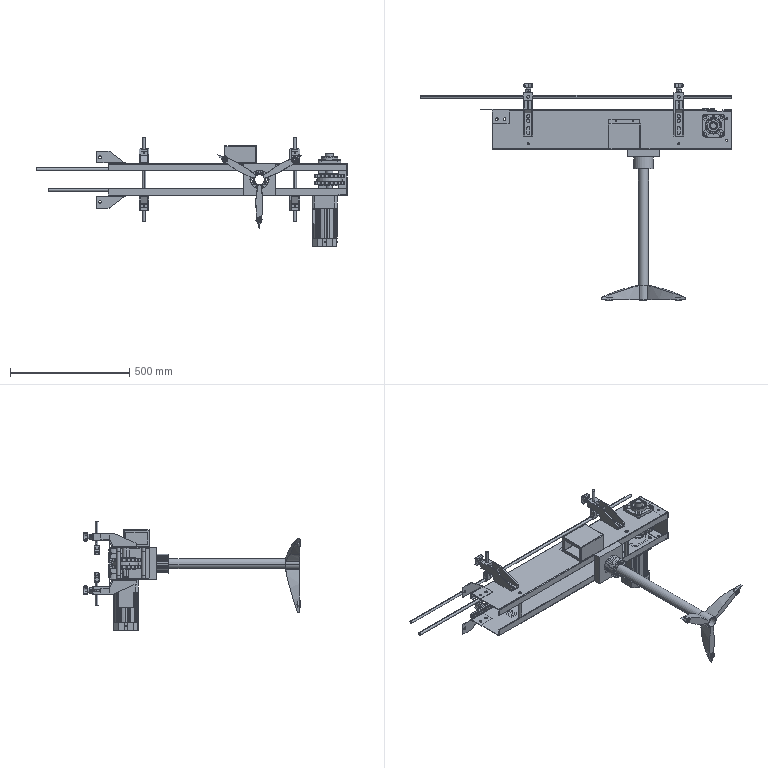Part | SolidWorks | 42 solids | 2324 faces | box 1300 x 909.194 x 459 mm | volume 5786853 mm3 | cylinder 1065 | plane 950 | spline 216 | cone 93 | commonest cylinder face diameters 2 x132 0.4 x102 6 x67 14 x60 1 x55 8.5 x48